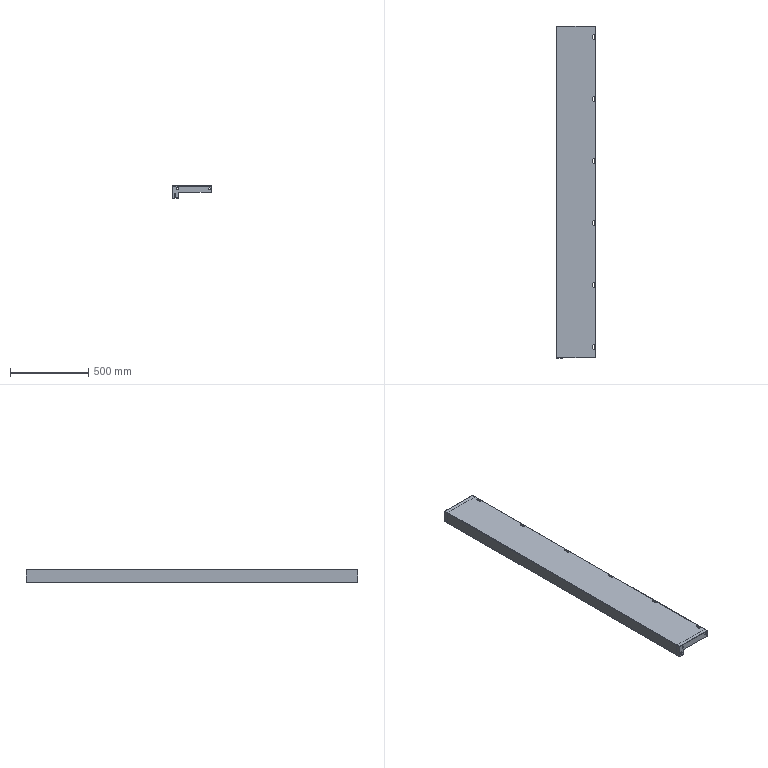Part | SolidWorks | features MirrorCompFeat 1, ReferencePattern 1 | 3 solids | 206 faces | box 250 x 2116 x 80 mm | volume 1147542 mm3 | plane 126 | cylinder 80 | commonest cylinder face diameters 6.2 x28 9 x18 11 x10 3.4 x9 10 x6 1 x5